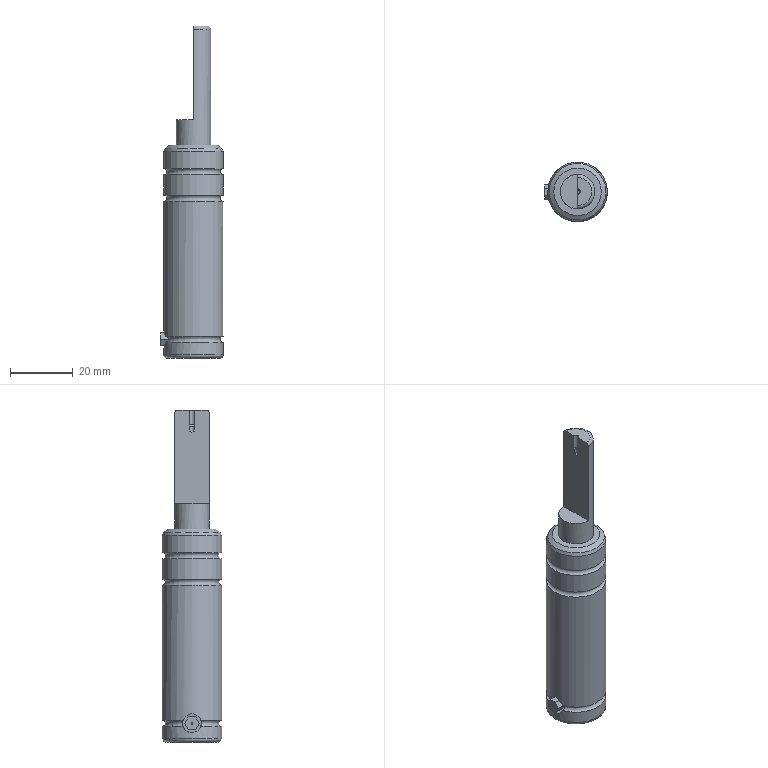Part | NX | features 1 2 | 1 solid | 36 faces | box 20 x 19 x 106 mm | volume 20839 mm3 | plane 14 | cylinder 11 | cone 6 | torus 5 | commonest cylinder face diameters 19 x4 6 x2 0.6 x1 1.558 x1 1.833 x1 5.1 x1
STEP:
#1=CARTESIAN_POINT('',(570.431,-100.172,-102.5));
#2=VERTEX_POINT('',#1);
#3=CARTESIAN_POINT('',(570.431,-100.172,-100.5));
#4=VERTEX_POINT('',#3);
#5=CARTESIAN_POINT('',(570.431,-100.172,-102.5));
#6=CARTESIAN_POINT('',(570.711,-100.172,-102.5));
#7=CARTESIAN_POINT('',(571.253,-100.089,-102.303));
#8=CARTESIAN_POINT('',(571.694,-99.956,-101.501));
#9=CARTESIAN_POINT('',(571.254,-100.089,-100.697));
#10=CARTESIAN_POINT('',(570.711,-100.172,-100.5));
#11=CARTESIAN_POINT('',(570.431,-100.172,-100.5));
#12=B_SPLINE_CURVE_WITH_KNOTS('',3,(#5,#6,#7,#8,#9,#10,#11),.UNSPECIFIED.,.F.,.F.,(4,1,1,1,4),(0.,0.0008273,0.001655,0.002482,0.003309),.UNSPECIFIED.);
#13=EDGE_CURVE('',#2,#4,#12,.T.);
#14=ORIENTED_EDGE('',*,*,#13,.T.);
#15=CARTESIAN_POINT('',(570.431,-105.828,-100.5));
#16=VERTEX_POINT('',#15);
#17=CARTESIAN_POINT('',(579.5,-103.,-100.5));
#18=DIRECTION('',(0.,0.,1.));
#19=DIRECTION('',(-1.,0.,0.));
#20=AXIS2_PLACEMENT_3D('',#17,#18,#19);
#21=CIRCLE('',#20,9.5);
#22=EDGE_CURVE('',#16,#4,#21,.T.);
#23=ORIENTED_EDGE('',*,*,#22,.F.);
#24=CARTESIAN_POINT('',(570.431,-105.828,-102.5));
#25=VERTEX_POINT('',#24);
#26=CARTESIAN_POINT('',(570.431,-105.828,-100.5));
#27=CARTESIAN_POINT('',(570.711,-105.828,-100.5));
#28=CARTESIAN_POINT('',(571.253,-105.911,-100.697));
#29=CARTESIAN_POINT('',(571.694,-106.044,-101.499));
#30=CARTESIAN_POINT('',(571.254,-105.911,-102.303));
#31=CARTESIAN_POINT('',(570.711,-105.828,-102.5));
#32=CARTESIAN_POINT('',(570.431,-105.828,-102.5));
#33=B_SPLINE_CURVE_WITH_KNOTS('',3,(#26,#27,#28,#29,#30,#31,#32),.UNSPECIFIED.,.F.,.F.,(4,1,1,1,4),(-0.001658,-0.0008295,-0.000000739,0.000828,0.001657),.UNSPECIFIED.);
#34=EDGE_CURVE('',#16,#25,#33,.T.);
#35=ORIENTED_EDGE('',*,*,#34,.T.);
#36=CARTESIAN_POINT('',(579.5,-103.,-102.5));
#37=DIRECTION('',(0.,0.,-1.));
#38=DIRECTION('',(-1.,0.,0.));
#39=AXIS2_PLACEMENT_3D('',#36,#37,#38);
#40=CIRCLE('',#39,9.5);
#41=EDGE_CURVE('',#2,#25,#40,.T.);
#42=ORIENTED_EDGE('',*,*,#41,.F.);
#43=EDGE_LOOP('',(#14,#23,#35,#42));
#44=FACE_BOUND('',#43,.T.);
#45=CARTESIAN_POINT('',(579.5,-103.,-101.5));
#46=DIRECTION('',(0.,0.,1.));
#47=DIRECTION('',(1.,0.,0.));
#48=AXIS2_PLACEMENT_3D('',#45,#46,#47);
#49=TOROIDAL_SURFACE('',#48,9.5,1.);
#50=ADVANCED_FACE('',(#44),#49,.F.);
#51=CARTESIAN_POINT('',(570.,-103.,-55.5));
#52=VERTEX_POINT('',#51);
#53=CARTESIAN_POINT('',(579.5,-103.,-55.5));
#54=DIRECTION('',(0.,0.,1.));
#55=DIRECTION('',(-1.,0.,0.));
#56=AXIS2_PLACEMENT_3D('',#53,#54,#55);
#57=CIRCLE('',#56,9.5);
#58=EDGE_CURVE('',#52,#52,#57,.T.);
#59=ORIENTED_EDGE('',*,*,#58,.F.);
#60=EDGE_LOOP('',(#59));
#61=FACE_BOUND('',#60,.T.);
#62=CARTESIAN_POINT('',(570.,-103.,-57.5));
#63=VERTEX_POINT('',#62);
#64=CARTESIAN_POINT('',(579.5,-103.,-57.5));
#65=DIRECTION('',(0.,0.,-1.));
#66=DIRECTION('',(-1.,0.,0.));
#67=AXIS2_PLACEMENT_3D('',#64,#65,#66);
#68=CIRCLE('',#67,9.5);
#69=EDGE_CURVE('',#63,#63,#68,.T.);
#70=ORIENTED_EDGE('',*,*,#69,.F.);
#71=EDGE_LOOP('',(#70));
#72=FACE_BOUND('',#71,.T.);
#73=CARTESIAN_POINT('',(579.5,-103.,-56.5));
#74=DIRECTION('',(0.,0.,1.));
#75=DIRECTION('',(1.,0.,0.));
#76=AXIS2_PLACEMENT_3D('',#73,#74,#75);
#77=TOROIDAL_SURFACE('',#76,9.5,1.);
#78=ADVANCED_FACE('',(#61,#72),#77,.F.);
#79=CARTESIAN_POINT('',(570.,-103.,-47.));
#80=VERTEX_POINT('',#79);
#81=CARTESIAN_POINT('',(579.5,-103.,-47.));
#82=DIRECTION('',(0.,0.,1.));
#83=DIRECTION('',(-1.,0.,0.));
#84=AXIS2_PLACEMENT_3D('',#81,#82,#83);
#85=CIRCLE('',#84,9.5);
#86=EDGE_CURVE('',#80,#80,#85,.T.);
#87=ORIENTED_EDGE('',*,*,#86,.F.);
#88=EDGE_LOOP('',(#87));
#89=FACE_BOUND('',#88,.T.);
#90=CARTESIAN_POINT('',(570.,-103.,-49.));
#91=VERTEX_POINT('',#90);
#92=CARTESIAN_POINT('',(579.5,-103.,-49.));
#93=DIRECTION('',(0.,0.,-1.));
#94=DIRECTION('',(-1.,0.,0.));
#95=AXIS2_PLACEMENT_3D('',#92,#93,#94);
#96=CIRCLE('',#95,9.5);
#97=EDGE_CURVE('',#91,#91,#96,.T.);
#98=ORIENTED_EDGE('',*,*,#97,.F.);
#99=EDGE_LOOP('',(#98));
#100=FACE_BOUND('',#99,.T.);
#101=CARTESIAN_POINT('',(579.5,-103.,-48.));
#102=DIRECTION('',(0.,0.,1.));
#103=DIRECTION('',(1.,0.,0.));
#104=AXIS2_PLACEMENT_3D('',#101,#102,#103);
#105=TOROIDAL_SURFACE('',#104,9.5,1.);
#106=ADVANCED_FACE('',(#89,#100),#105,.F.);
#107=ORIENTED_EDGE('',*,*,#86,.T.);
#108=EDGE_LOOP('',(#107));
#109=FACE_BOUND('',#108,.T.);
#110=CARTESIAN_POINT('',(570.,-103.,-41.5));
#111=VERTEX_POINT('',#110);
#112=CARTESIAN_POINT('',(579.5,-103.,-41.5));
#113=DIRECTION('',(0.,0.,1.));
#114=DIRECTION('',(-1.,0.,0.));
#115=AXIS2_PLACEMENT_3D('',#112,#113,#114);
#116=CIRCLE('',#115,9.5);
#117=EDGE_CURVE('',#111,#111,#116,.T.);
#118=ORIENTED_EDGE('',*,*,#117,.F.);
#119=EDGE_LOOP('',(#118));
#120=FACE_BOUND('',#119,.T.);
#121=CARTESIAN_POINT('',(579.5,-103.,-74.5));
#122=DIRECTION('',(0.,0.,1.));
#123=DIRECTION('',(1.,0.,0.));
#124=AXIS2_PLACEMENT_3D('',#121,#122,#123);
#125=CYLINDRICAL_SURFACE('',#124,9.5);
#126=ADVANCED_FACE('',(#109,#120),#125,.T.);
#127=ORIENTED_EDGE('',*,*,#117,.T.);
#128=EDGE_LOOP('',(#127));
#129=FACE_BOUND('',#128,.T.);
#130=CARTESIAN_POINT('',(570.452,-103.,-40.5));
#131=VERTEX_POINT('',#130);
#132=CARTESIAN_POINT('',(579.5,-103.,-40.5));
#133=DIRECTION('',(0.,0.,1.));
#134=DIRECTION('',(-1.,0.,0.));
#135=AXIS2_PLACEMENT_3D('',#132,#133,#134);
#136=CIRCLE('',#135,9.048);
#137=EDGE_CURVE('',#131,#131,#136,.T.);
#138=ORIENTED_EDGE('',*,*,#137,.F.);
#139=EDGE_LOOP('',(#138));
#140=FACE_BOUND('',#139,.T.);
#141=CARTESIAN_POINT('',(579.5,-103.,-41.));
#142=DIRECTION('',(0.,0.,-1.));
#143=DIRECTION('',(1.,0.,0.));
#144=AXIS2_PLACEMENT_3D('',#141,#142,#143);
#145=CONICAL_SURFACE('',#144,9.274,0.4248);
#146=ADVANCED_FACE('',(#129,#140),#145,.T.);
#147=ORIENTED_EDGE('',*,*,#137,.T.);
#148=EDGE_LOOP('',(#147));
#149=FACE_BOUND('',#148,.T.);
#150=CARTESIAN_POINT('',(571.9,-103.,-39.5));
#151=VERTEX_POINT('',#150);
#152=CARTESIAN_POINT('',(579.5,-103.,-39.5));
#153=DIRECTION('',(0.,0.,1.));
#154=DIRECTION('',(-1.,0.,0.));
#155=AXIS2_PLACEMENT_3D('',#152,#153,#154);
#156=CIRCLE('',#155,7.6);
#157=EDGE_CURVE('',#151,#151,#156,.T.);
#158=ORIENTED_EDGE('',*,*,#157,.F.);
#159=EDGE_LOOP('',(#158));
#160=FACE_BOUND('',#159,.T.);
#161=CARTESIAN_POINT('',(579.5,-103.,-40.));
#162=DIRECTION('',(0.,0.,-1.));
#163=DIRECTION('',(1.,0.,0.));
#164=AXIS2_PLACEMENT_3D('',#161,#162,#163);
#165=CONICAL_SURFACE('',#164,8.324,0.9663);
#166=ADVANCED_FACE('',(#149,#160),#165,.T.);
#167=ORIENTED_EDGE('',*,*,#22,.T.);
#168=CARTESIAN_POINT('',(570.431,-100.172,-100.5));
#169=CARTESIAN_POINT('',(570.366,-100.379,-99.913));
#170=CARTESIAN_POINT('',(570.138,-101.142,-98.904));
#171=CARTESIAN_POINT('',(569.931,-103.001,-98.299));
#172=CARTESIAN_POINT('',(570.136,-104.85,-98.899));
#173=CARTESIAN_POINT('',(570.366,-105.621,-99.913));
#174=CARTESIAN_POINT('',(570.431,-105.828,-100.5));
#175=B_SPLINE_CURVE_WITH_KNOTS('',3,(#168,#169,#170,#171,#172,#173,#174),.UNSPECIFIED.,.F.,.F.,(4,1,1,1,4),(-0.003701,-0.001851,-0.000000566,0.00185,0.0037),.UNSPECIFIED.);
#176=EDGE_CURVE('',#4,#16,#175,.T.);
#177=ORIENTED_EDGE('',*,*,#176,.T.);
#178=EDGE_LOOP('',(#167,#177));
#179=FACE_BOUND('',#178,.T.);
#180=ORIENTED_EDGE('',*,*,#69,.T.);
#181=EDGE_LOOP('',(#180));
#182=FACE_BOUND('',#181,.T.);
#183=CARTESIAN_POINT('',(579.5,-103.,-74.5));
#184=DIRECTION('',(0.,0.,1.));
#185=DIRECTION('',(1.,0.,0.));
#186=AXIS2_PLACEMENT_3D('',#183,#184,#185);
#187=CYLINDRICAL_SURFACE('',#186,9.5);
#188=ADVANCED_FACE('',(#179,#182),#187,.T.);
#189=ORIENTED_EDGE('',*,*,#58,.T.);
#190=EDGE_LOOP('',(#189));
#191=FACE_BOUND('',#190,.T.);
#192=ORIENTED_EDGE('',*,*,#97,.T.);
#193=EDGE_LOOP('',(#192));
#194=FACE_BOUND('',#193,.T.);
#195=CARTESIAN_POINT('',(579.5,-103.,-74.5));
#196=DIRECTION('',(0.,0.,1.));
#197=DIRECTION('',(1.,0.,0.));
#198=AXIS2_PLACEMENT_3D('',#195,#196,#197);
#199=CYLINDRICAL_SURFACE('',#198,9.5);
#200=ADVANCED_FACE('',(#191,#194),#199,.T.);
#201=CARTESIAN_POINT('',(579.5,-102.083,-6.25));
#202=VERTEX_POINT('',#201);
#203=CARTESIAN_POINT('',(579.5,-103.917,-6.25));
#204=VERTEX_POINT('',#203);
#205=CARTESIAN_POINT('',(579.5,-103.,-6.25));
#206=DIRECTION('',(0.,0.,-1.));
#207=DIRECTION('',(-1.,0.,0.));
#208=AXIS2_PLACEMENT_3D('',#205,#206,#207);
#209=CIRCLE('',#208,0.9167);
#210=EDGE_CURVE('',#202,#204,#209,.T.);
#211=ORIENTED_EDGE('',*,*,#210,.T.);
#212=CARTESIAN_POINT('',(579.5,-103.917,-1.5));
#213=VERTEX_POINT('',#212);
#214=CARTESIAN_POINT('',(579.5,-103.917,-3.875));
#215=DIRECTION('',(0.,0.,-1.));
#216=VECTOR('',#215,1000.);
#217=LINE('',#214,#216);
#218=EDGE_CURVE('',#204,#213,#217,.F.);
#219=ORIENTED_EDGE('',*,*,#218,.T.);
#220=CARTESIAN_POINT('',(579.5,-102.083,-1.5));
#221=VERTEX_POINT('',#220);
#222=CARTESIAN_POINT('',(579.5,-103.,-1.5));
#223=DIRECTION('',(0.,0.,-1.));
#224=DIRECTION('',(-1.,0.,0.));
#225=AXIS2_PLACEMENT_3D('',#222,#223,#224);
#226=CIRCLE('',#225,0.9167);
#227=EDGE_CURVE('',#221,#213,#226,.T.);
#228=ORIENTED_EDGE('',*,*,#227,.F.);
#229=CARTESIAN_POINT('',(579.5,-102.083,-3.875));
#230=DIRECTION('',(0.,0.,-1.));
#231=VECTOR('',#230,1000.);
#232=LINE('',#229,#231);
#233=EDGE_CURVE('',#221,#202,#232,.T.);
#234=ORIENTED_EDGE('',*,*,#233,.T.);
#235=EDGE_LOOP('',(#211,#219,#228,#234));
#236=FACE_BOUND('',#235,.T.);
#237=CARTESIAN_POINT('',(579.5,-103.,-3.875));
#238=DIRECTION('',(0.,0.,-1.));
#239=DIRECTION('',(1.,0.,0.));
#240=AXIS2_PLACEMENT_3D('',#237,#238,#239);
#241=CYLINDRICAL_SURFACE('',#240,0.9167);
#242=ADVANCED_FACE('',(#236),#241,.F.);
#243=ORIENTED_EDGE('',*,*,#210,.F.);
#244=CARTESIAN_POINT('',(579.5,-102.221,-6.75));
#245=VERTEX_POINT('',#244);
#246=CARTESIAN_POINT('',(579.5,-103.,-9.583));
#247=DIRECTION('',(0.,0.2652,0.9642));
#248=VECTOR('',#247,1000.);
#249=LINE('',#246,#248);
#250=EDGE_CURVE('',#202,#245,#249,.F.);
#251=ORIENTED_EDGE('',*,*,#250,.T.);
#252=CARTESIAN_POINT('',(579.5,-103.779,-6.75));
#253=VERTEX_POINT('',#252);
#254=CARTESIAN_POINT('',(579.5,-103.,-6.75));
#255=DIRECTION('',(0.,0.,-1.));
#256=DIRECTION('',(-1.,0.,0.));
#257=AXIS2_PLACEMENT_3D('',#254,#255,#256);
#258=CIRCLE('',#257,0.7792);
#259=EDGE_CURVE('',#245,#253,#258,.T.);
#260=ORIENTED_EDGE('',*,*,#259,.T.);
#261=CARTESIAN_POINT('',(579.5,-103.,-9.583));
#262=DIRECTION('',(0.,0.2652,-0.9642));
#263=VECTOR('',#262,1000.);
#264=LINE('',#261,#263);
#265=EDGE_CURVE('',#253,#204,#264,.F.);
#266=ORIENTED_EDGE('',*,*,#265,.T.);
#267=EDGE_LOOP('',(#243,#251,#260,#266));
#268=FACE_BOUND('',#267,.T.);
#269=CARTESIAN_POINT('',(579.5,-103.,-6.5));
#270=DIRECTION('',(0.,0.,1.));
#271=DIRECTION('',(1.,0.,0.));
#272=AXIS2_PLACEMENT_3D('',#269,#270,#271);
#273=CONICAL_SURFACE('',#272,0.8479,0.2684);
#274=ADVANCED_FACE('',(#268),#273,.F.);
#275=CARTESIAN_POINT('',(579.5,-102.221,-8.25));
#276=VERTEX_POINT('',#275);
#277=CARTESIAN_POINT('',(579.5,-103.779,-8.25));
#278=VERTEX_POINT('',#277);
#279=CARTESIAN_POINT('',(579.5,-103.,-8.25));
#280=DIRECTION('',(0.,0.,-1.));
#281=DIRECTION('',(-1.,0.,0.));
#282=AXIS2_PLACEMENT_3D('',#279,#280,#281);
#283=CIRCLE('',#282,0.7792);
#284=EDGE_CURVE('',#276,#278,#283,.T.);
#285=ORIENTED_EDGE('',*,*,#284,.T.);
#286=CARTESIAN_POINT('',(579.5,-103.779,-7.5));
#287=DIRECTION('',(0.,0.,-1.));
#288=VECTOR('',#287,1000.);
#289=LINE('',#286,#288);
#290=EDGE_CURVE('',#278,#253,#289,.F.);
#291=ORIENTED_EDGE('',*,*,#290,.T.);
#292=ORIENTED_EDGE('',*,*,#259,.F.);
#293=CARTESIAN_POINT('',(579.5,-102.221,-7.5));
#294=DIRECTION('',(0.,0.,-1.));
#295=VECTOR('',#294,1000.);
#296=LINE('',#293,#295);
#297=EDGE_CURVE('',#245,#276,#296,.T.);
#298=ORIENTED_EDGE('',*,*,#297,.T.);
#299=EDGE_LOOP('',(#285,#291,#292,#298));
#300=FACE_BOUND('',#299,.T.);
#301=CARTESIAN_POINT('',(579.5,-103.,-7.5));
#302=DIRECTION('',(0.,0.,-1.));
#303=DIRECTION('',(1.,0.,0.));
#304=AXIS2_PLACEMENT_3D('',#301,#302,#303);
#305=CYLINDRICAL_SURFACE('',#304,0.7792);
#306=ADVANCED_FACE('',(#300),#305,.F.);
#307=ORIENTED_EDGE('',*,*,#284,.F.);
#308=CARTESIAN_POINT('',(579.5,-103.,-8.718));
#309=VERTEX_POINT('',#308);
#310=CARTESIAN_POINT('',(579.5,-103.,-8.718));
#311=DIRECTION('',(0.,0.8572,0.515));
#312=VECTOR('',#311,1000.);
#313=LINE('',#310,#312);
#314=EDGE_CURVE('',#276,#309,#313,.F.);
#315=ORIENTED_EDGE('',*,*,#314,.T.);
#316=CARTESIAN_POINT('',(579.5,-103.,-8.718));
#317=DIRECTION('',(0.,0.8572,-0.515));
#318=VECTOR('',#317,1000.);
#319=LINE('',#316,#318);
#320=EDGE_CURVE('',#309,#278,#319,.F.);
#321=ORIENTED_EDGE('',*,*,#320,.T.);
#322=EDGE_LOOP('',(#307,#315,#321));
#323=FACE_BOUND('',#322,.T.);
#324=CARTESIAN_POINT('',(579.5,-103.,-8.484));
#325=DIRECTION('',(0.,0.,1.));
#326=DIRECTION('',(1.,0.,0.));
#327=AXIS2_PLACEMENT_3D('',#324,#325,#326);
#328=CONICAL_SURFACE('',#327,0.3896,1.03);
#329=ADVANCED_FACE('',(#323),#328,.F.);
#330=CARTESIAN_POINT('',(576.5,-103.,-101.5));
#331=VERTEX_POINT('',#330);
#332=CARTESIAN_POINT('',(579.5,-103.,-101.5));
#333=DIRECTION('',(0.,0.,1.));
#334=DIRECTION('',(-1.,0.,0.));
#335=AXIS2_PLACEMENT_3D('',#332,#333,#334);
#336=CIRCLE('',#335,3.);
#337=EDGE_CURVE('',#331,#331,#336,.T.);
#338=ORIENTED_EDGE('',*,*,#337,.T.);
#339=EDGE_LOOP('',(#338));
#340=FACE_BOUND('',#339,.T.);
#341=CARTESIAN_POINT('',(576.5,-103.,-107.5));
#342=VERTEX_POINT('',#341);
#343=CARTESIAN_POINT('',(579.5,-103.,-107.5));
#344=DIRECTION('',(0.,0.,1.));
#345=DIRECTION('',(-1.,0.,0.));
#346=AXIS2_PLACEMENT_3D('',#343,#344,#345);
#347=CIRCLE('',#346,3.);
#348=EDGE_CURVE('',#342,#342,#347,.T.);
#349=ORIENTED_EDGE('',*,*,#348,.F.);
#350=EDGE_LOOP('',(#349));
#351=FACE_BOUND('',#350,.T.);
#352=CARTESIAN_POINT('',(579.5,-103.,-104.5));
#353=DIRECTION('',(0.,0.,1.));
#354=DIRECTION('',(1.,0.,0.));
#355=AXIS2_PLACEMENT_3D('',#352,#353,#354);
#356=CYLINDRICAL_SURFACE('',#355,3.);
#357=ADVANCED_FACE('',(#340,#351),#356,.F.);
#358=CARTESIAN_POINT('',(576.95,-103.,-101.));
#359=VERTEX_POINT('',#358);
#360=CARTESIAN_POINT('',(579.5,-103.,-101.));
#361=DIRECTION('',(0.,0.,1.));
#362=DIRECTION('',(-1.,0.,0.));
#363=AXIS2_PLACEMENT_3D('',#360,#361,#362);
#364=CIRCLE('',#363,2.55);
#365=EDGE_CURVE('',#359,#359,#364,.T.);
#366=ORIENTED_EDGE('',*,*,#365,.T.);
#367=EDGE_LOOP('',(#366));
#368=FACE_BOUND('',#367,.T.);
#369=ORIENTED_EDGE('',*,*,#337,.F.);
#370=EDGE_LOOP('',(#369));
#371=FACE_BOUND('',#370,.T.);
#372=CARTESIAN_POINT('',(579.5,-103.,-101.25));
#373=DIRECTION('',(0.,0.,-1.));
#374=DIRECTION('',(1.,0.,0.));
#375=AXIS2_PLACEMENT_3D('',#372,#373,#374);
#376=CONICAL_SURFACE('',#375,2.775,0.7328);
#377=ADVANCED_FACE('',(#368,#371),#376,.F.);
#378=CARTESIAN_POINT('',(576.95,-103.,-99.5));
#379=VERTEX_POINT('',#378);
#380=CARTESIAN_POINT('',(579.5,-103.,-99.5));
#381=DIRECTION('',(0.,0.,1.));
#382=DIRECTION('',(-1.,0.,0.));
#383=AXIS2_PLACEMENT_3D('',#380,#381,#382);
#384=CIRCLE('',#383,2.55);
#385=EDGE_CURVE('',#379,#379,#384,.T.);
#386=ORIENTED_EDGE('',*,*,#385,.T.);
#387=EDGE_LOOP('',(#386));
#388=FACE_BOUND('',#387,.T.);
#389=ORIENTED_EDGE('',*,*,#365,.F.);
#390=EDGE_LOOP('',(#389));
#391=FACE_BOUND('',#390,.T.);
#392=CARTESIAN_POINT('',(579.5,-103.,-100.25));
#393=DIRECTION('',(0.,0.,1.));
#394=DIRECTION('',(1.,0.,0.));
#395=AXIS2_PLACEMENT_3D('',#392,#393,#394);
#396=CYLINDRICAL_SURFACE('',#395,2.55);
#397=ADVANCED_FACE('',(#388,#391),#396,.F.);
#398=ORIENTED_EDGE('',*,*,#385,.F.);
#399=EDGE_LOOP('',(#398));
#400=FACE_BOUND('',#399,.T.);
#401=CARTESIAN_POINT('',(579.5,-103.,-97.968));
#402=VERTEX_POINT('',#401);
#403=VERTEX_LOOP('',#402);
#404=FACE_BOUND('',#403,.T.);
#405=CARTESIAN_POINT('',(579.5,-103.,-98.734));
#406=DIRECTION('',(0.,0.,-1.));
#407=DIRECTION('',(1.,0.,0.));
#408=AXIS2_PLACEMENT_3D('',#405,#406,#407);
#409=CONICAL_SURFACE('',#408,1.275,1.03);
#410=ADVANCED_FACE('',(#400,#404),#409,.F.);
#411=CARTESIAN_POINT('',(579.5,-97.5,-2.5));
#412=VERTEX_POINT('',#411);
#413=CARTESIAN_POINT('',(579.5,-97.5,-31.5));
#414=VERTEX_POINT('',#413);
#415=CARTESIAN_POINT('',(579.5,-97.5,-20.5));
#416=DIRECTION('',(0.,0.,1.));
#417=VECTOR('',#416,1000.);
#418=LINE('',#415,#417);
#419=EDGE_CURVE('',#412,#414,#418,.F.);
#420=ORIENTED_EDGE('',*,*,#419,.F.);
#421=CARTESIAN_POINT('',(579.5,-108.5,-2.5));
#422=VERTEX_POINT('',#421);
#423=CARTESIAN_POINT('',(579.5,-103.,-2.5));
#424=DIRECTION('',(0.,0.,1.));
#425=DIRECTION('',(1.,0.,0.));
#426=AXIS2_PLACEMENT_3D('',#423,#424,#425);
#427=CIRCLE('',#426,5.5);
#428=EDGE_CURVE('',#422,#412,#427,.T.);
#429=ORIENTED_EDGE('',*,*,#428,.F.);
#430=CARTESIAN_POINT('',(579.5,-108.5,-31.5));
#431=VERTEX_POINT('',#430);
#432=CARTESIAN_POINT('',(579.5,-108.5,-20.5));
#433=DIRECTION('',(0.,0.,1.));
#434=VECTOR('',#433,1000.);
#435=LINE('',#432,#434);
#436=EDGE_CURVE('',#431,#422,#435,.T.);
#437=ORIENTED_EDGE('',*,*,#436,.F.);
#438=CARTESIAN_POINT('',(579.5,-103.,-31.5));
#439=DIRECTION('',(0.,0.,-1.));
#440=DIRECTION('',(-1.,0.,0.));
#441=AXIS2_PLACEMENT_3D('',#438,#439,#440);
#442=CIRCLE('',#441,5.5);
#443=EDGE_CURVE('',#414,#431,#442,.F.);
#444=ORIENTED_EDGE('',*,*,#443,.F.);
#445=EDGE_LOOP('',(#420,#429,#437,#444));
#446=FACE_BOUND('',#445,.T.);
#447=CARTESIAN_POINT('',(574.,-103.,-39.5));
#448=VERTEX_POINT('',#447);
#449=CARTESIAN_POINT('',(579.5,-103.,-39.5));
#450=DIRECTION('',(0.,0.,-1.));
#451=DIRECTION('',(-1.,0.,0.));
#452=AXIS2_PLACEMENT_3D('',#449,#450,#451);
#453=CIRCLE('',#452,5.5);
#454=EDGE_CURVE('',#448,#448,#453,.T.);
#455=ORIENTED_EDGE('',*,*,#454,.F.);
#456=EDGE_LOOP('',(#455));
#457=FACE_BOUND('',#456,.T.);
#458=CARTESIAN_POINT('',(579.5,-103.,-20.5));
#459=DIRECTION('',(0.,0.,1.));
#460=DIRECTION('',(1.,0.,0.));
#461=AXIS2_PLACEMENT_3D('',#458,#459,#460);
#462=CYLINDRICAL_SURFACE('',#461,5.5);
#463=ADVANCED_FACE('',(#446,#457),#462,.T.);
#464=CARTESIAN_POINT('',(579.5,-98.5,-1.5));
#465=VERTEX_POINT('',#464);
#466=CARTESIAN_POINT('',(579.5,-98.5,-2.5));
#467=DIRECTION('',(1.,0.,0.));
#468=DIRECTION('',(0.,0.,-1.));
#469=AXIS2_PLACEMENT_3D('',#466,#467,#468);
#470=CIRCLE('',#469,1.);
#471=EDGE_CURVE('',#465,#412,#470,.F.);
#472=ORIENTED_EDGE('',*,*,#471,.F.);
#473=CARTESIAN_POINT('',(579.5,-107.5,-1.5));
#474=VERTEX_POINT('',#473);
#475=CARTESIAN_POINT('',(579.5,-103.,-1.5));
#476=DIRECTION('',(0.,0.,-1.));
#477=DIRECTION('',(1.,0.,0.));
#478=AXIS2_PLACEMENT_3D('',#475,#476,#477);
#479=CIRCLE('',#478,4.5);
#480=EDGE_CURVE('',#465,#474,#479,.T.);
#481=ORIENTED_EDGE('',*,*,#480,.T.);
#482=CARTESIAN_POINT('',(579.5,-107.5,-2.5));
#483=DIRECTION('',(1.,0.,0.));
#484=DIRECTION('',(0.,0.,-1.));
#485=AXIS2_PLACEMENT_3D('',#482,#483,#484);
#486=CIRCLE('',#485,1.);
#487=EDGE_CURVE('',#422,#474,#486,.F.);
#488=ORIENTED_EDGE('',*,*,#487,.F.);
#489=ORIENTED_EDGE('',*,*,#428,.T.);
#490=EDGE_LOOP('',(#472,#481,#488,#489));
#491=FACE_BOUND('',#490,.T.);
#492=CARTESIAN_POINT('',(579.5,-103.,-2.5));
#493=DIRECTION('',(0.,0.,1.));
#494=DIRECTION('',(1.,0.,0.));
#495=AXIS2_PLACEMENT_3D('',#492,#493,#494);
#496=TOROIDAL_SURFACE('',#495,4.5,1.);
#497=ADVANCED_FACE('',(#491),#496,.T.);
#498=CARTESIAN_POINT('',(589.,-103.,-106.5));
#499=VERTEX_POINT('',#498);
#500=CARTESIAN_POINT('',(579.5,-103.,-106.5));
#501=DIRECTION('',(0.,0.,-1.));
#502=DIRECTION('',(1.,0.,0.));
#503=AXIS2_PLACEMENT_3D('',#500,#501,#502);
#504=CIRCLE('',#503,9.5);
#505=EDGE_CURVE('',#499,#499,#504,.T.);
#506=ORIENTED_EDGE('',*,*,#505,.T.);
#507=EDGE_LOOP('',(#506));
#508=FACE_BOUND('',#507,.T.);
#509=CARTESIAN_POINT('',(588.,-103.,-107.5));
#510=VERTEX_POINT('',#509);
#511=CARTESIAN_POINT('',(579.5,-103.,-107.5));
#512=DIRECTION('',(0.,0.,1.));
#513=DIRECTION('',(1.,0.,0.));
#514=AXIS2_PLACEMENT_3D('',#511,#512,#513);
#515=CIRCLE('',#514,8.5);
#516=EDGE_CURVE('',#510,#510,#515,.T.);
#517=ORIENTED_EDGE('',*,*,#516,.T.);
#518=EDGE_LOOP('',(#517));
#519=FACE_BOUND('',#518,.T.);
#520=CARTESIAN_POINT('',(579.5,-103.,-106.5));
#521=DIRECTION('',(0.,0.,-1.));
#522=DIRECTION('',(-1.,0.,0.));
#523=AXIS2_PLACEMENT_3D('',#520,#521,#522);
#524=TOROIDAL_SURFACE('',#523,8.5,1.);
#525=ADVANCED_FACE('',(#508,#519),#524,.T.);
#526=ORIENTED_EDGE('',*,*,#505,.F.);
#527=EDGE_LOOP('',(#526));
#528=FACE_BOUND('',#527,.T.);
#529=CARTESIAN_POINT('',(570.431,-105.828,-102.5));
#530=CARTESIAN_POINT('',(570.366,-105.621,-103.087));
#531=CARTESIAN_POINT('',(570.138,-104.858,-104.096));
#532=CARTESIAN_POINT('',(569.931,-102.999,-104.701));
#533=CARTESIAN_POINT('',(570.136,-101.15,-104.101));
#534=CARTESIAN_POINT('',(570.366,-100.379,-103.087));
#535=CARTESIAN_POINT('',(570.431,-100.172,-102.5));
#536=B_SPLINE_CURVE_WITH_KNOTS('',3,(#529,#530,#531,#532,#533,#534,#535),.UNSPECIFIED.,.F.,.F.,(4,1,1,1,4),(0.,0.00185,0.0037,0.005549,0.007399),.UNSPECIFIED.);
#537=EDGE_CURVE('',#25,#2,#536,.T.);
#538=ORIENTED_EDGE('',*,*,#537,.T.);
#539=ORIENTED_EDGE('',*,*,#41,.T.);
#540=EDGE_LOOP('',(#538,#539));
#541=FACE_BOUND('',#540,.T.);
#542=CARTESIAN_POINT('',(579.5,-103.,-74.5));
#543=DIRECTION('',(0.,0.,1.));
#544=DIRECTION('',(1.,0.,0.));
#545=AXIS2_PLACEMENT_3D('',#542,#543,#544);
#546=CYLINDRICAL_SURFACE('',#545,9.5);
#547=ADVANCED_FACE('',(#528,#541),#546,.T.);
#548=CARTESIAN_POINT('',(574.,-103.,-98.5));
#549=VERTEX_POINT('',#548);
#550=CARTESIAN_POINT('',(574.,-103.,-101.5));
#551=DIRECTION('',(1.,0.,0.));
#552=DIRECTION('',(0.,0.,1.));
#553=AXIS2_PLACEMENT_3D('',#550,#551,#552);
#554=CIRCLE('',#553,3.);
#555=EDGE_CURVE('',#549,#549,#554,.T.);
#556=ORIENTED_EDGE('',*,*,#555,.T.);
#557=EDGE_LOOP('',(#556));
#558=FACE_BOUND('',#557,.T.);
#559=ORIENTED_EDGE('',*,*,#176,.F.);
#560=ORIENTED_EDGE('',*,*,#13,.F.);
#561=ORIENTED_EDGE('',*,*,#537,.F.);
#562=ORIENTED_EDGE('',*,*,#34,.F.);
#563=EDGE_LOOP('',(#559,#560,#561,#562));
#564=FACE_BOUND('',#563,.T.);
#565=CARTESIAN_POINT('',(572.,-103.,-101.5));
#566=DIRECTION('',(1.,0.,0.));
#567=DIRECTION('',(0.,0.,-1.));
#568=AXIS2_PLACEMENT_3D('',#565,#566,#567);
#569=CYLINDRICAL_SURFACE('',#568,3.);
#570=ADVANCED_FACE('',(#558,#564),#569,.F.);
#571=CARTESIAN_POINT('',(574.,-103.,-101.2));
#572=VERTEX_POINT('',#571);
#573=CARTESIAN_POINT('',(574.,-103.,-101.5));
#574=DIRECTION('',(1.,0.,0.));
#575=DIRECTION('',(0.,0.,1.));
#576=AXIS2_PLACEMENT_3D('',#573,#574,#575);
#577=CIRCLE('',#576,0.3);
#578=EDGE_CURVE('',#572,#572,#577,.T.);
#579=ORIENTED_EDGE('',*,*,#578,.T.);
#580=EDGE_LOOP('',(#579));
#581=FACE_BOUND('',#580,.T.);
#582=CARTESIAN_POINT('',(569.,-103.,-101.2));
#583=VERTEX_POINT('',#582);
#584=CARTESIAN_POINT('',(569.,-103.,-101.5));
#585=DIRECTION('',(1.,0.,0.));
#586=DIRECTION('',(0.,0.,1.));
#587=AXIS2_PLACEMENT_3D('',#584,#585,#586);
#588=CIRCLE('',#587,0.3);
#589=EDGE_CURVE('',#583,#583,#588,.T.);
#590=ORIENTED_EDGE('',*,*,#589,.F.);
#591=EDGE_LOOP('',(#590));
#592=FACE_BOUND('',#591,.T.);
#593=CARTESIAN_POINT('',(570.5,-103.,-101.5));
#594=DIRECTION('',(1.,0.,0.));
#595=DIRECTION('',(0.,0.,-1.));
#596=AXIS2_PLACEMENT_3D('',#593,#594,#595);
#597=CYLINDRICAL_SURFACE('',#596,0.3);
#598=ADVANCED_FACE('',(#581,#592),#597,.F.);
#599=ORIENTED_EDGE('',*,*,#578,.F.);
#600=EDGE_LOOP('',(#599));
#601=FACE_BOUND('',#600,.T.);
#602=CARTESIAN_POINT('',(574.,-103.,-101.5));
#603=DIRECTION('',(1.,0.,0.));
#604=DIRECTION('',(0.,0.,-1.));
#605=AXIS2_PLACEMENT_3D('',#602,#603,#604);
#606=PLANE('',#605);
#607=ADVANCED_FACE('',(#601),#606,.F.);
#608=ORIENTED_EDGE('',*,*,#589,.T.);
#609=EDGE_LOOP('',(#608));
#610=FACE_BOUND('',#609,.T.);
#611=CARTESIAN_POINT('',(569.,-104.155,-99.5));
#612=VERTEX_POINT('',#611);
#613=CARTESIAN_POINT('',(569.,-101.845,-99.5));
#614=VERTEX_POINT('',#613);
#615=CARTESIAN_POINT('',(569.,-103.,-99.5));
#616=DIRECTION('',(0.,1.,0.));
#617=VECTOR('',#616,1000.);
#618=LINE('',#615,#617);
#619=EDGE_CURVE('',#612,#614,#618,.T.);
#620=ORIENTED_EDGE('',*,*,#619,.T.);
#621=CARTESIAN_POINT('',(569.,-100.691,-101.5));
#622=VERTEX_POINT('',#621);
#623=CARTESIAN_POINT('',(569.,-101.268,-100.5));
#624=DIRECTION('',(0.,0.5,-0.866));
#625=VECTOR('',#624,1000.);
#626=LINE('',#623,#625);
#627=EDGE_CURVE('',#614,#622,#626,.T.);
#628=ORIENTED_EDGE('',*,*,#627,.T.);
#629=CARTESIAN_POINT('',(569.,-101.845,-103.5));
#630=VERTEX_POINT('',#629);
#631=CARTESIAN_POINT('',(569.,-101.268,-102.5));
#632=DIRECTION('',(0.,-0.5,-0.866));
#633=VECTOR('',#632,1000.);
#634=LINE('',#631,#633);
#635=EDGE_CURVE('',#622,#630,#634,.T.);
#636=ORIENTED_EDGE('',*,*,#635,.T.);
#637=CARTESIAN_POINT('',(569.,-104.155,-103.5));
#638=VERTEX_POINT('',#637);
#639=CARTESIAN_POINT('',(569.,-103.,-103.5));
#640=DIRECTION('',(0.,-1.,0.));
#641=VECTOR('',#640,1000.);
#642=LINE('',#639,#641);
#643=EDGE_CURVE('',#630,#638,#642,.T.);
#644=ORIENTED_EDGE('',*,*,#643,.T.);
#645=CARTESIAN_POINT('',(569.,-105.309,-101.5));
#646=VERTEX_POINT('',#645);
#647=CARTESIAN_POINT('',(569.,-104.732,-102.5));
#648=DIRECTION('',(0.,-0.5,0.866));
#649=VECTOR('',#648,1000.);
#650=LINE('',#647,#649);
#651=EDGE_CURVE('',#638,#646,#650,.T.);
#652=ORIENTED_EDGE('',*,*,#651,.T.);
#653=CARTESIAN_POINT('',(569.,-104.732,-100.5));
#654=DIRECTION('',(0.,0.5,0.866));
#655=VECTOR('',#654,1000.);
#656=LINE('',#653,#655);
#657=EDGE_CURVE('',#646,#612,#656,.T.);
#658=ORIENTED_EDGE('',*,*,#657,.T.);
#659=EDGE_LOOP('',(#620,#628,#636,#644,#652,#658));
#660=FACE_BOUND('',#659,.T.);
#661=CARTESIAN_POINT('',(569.,-103.,-101.5));
#662=DIRECTION('',(-1.,0.,0.));
#663=DIRECTION('',(0.,0.,-1.));
#664=AXIS2_PLACEMENT_3D('',#661,#662,#663);
#665=PLANE('',#664);
#666=ADVANCED_FACE('',(#610,#660),#665,.T.);
#667=CARTESIAN_POINT('',(574.,-105.309,-101.5));
#668=VERTEX_POINT('',#667);
#669=CARTESIAN_POINT('',(571.5,-105.309,-101.5));
#670=DIRECTION('',(1.,0.,0.));
#671=VECTOR('',#670,1000.);
#672=LINE('',#669,#671);
#673=EDGE_CURVE('',#646,#668,#672,.T.);
#674=ORIENTED_EDGE('',*,*,#673,.T.);
#675=CARTESIAN_POINT('',(574.,-104.155,-99.5));
#676=VERTEX_POINT('',#675);
#677=CARTESIAN_POINT('',(574.,-104.732,-100.5));
#678=DIRECTION('',(0.,-0.5,-0.866));
#679=VECTOR('',#678,1000.);
#680=LINE('',#677,#679);
#681=EDGE_CURVE('',#676,#668,#680,.T.);
#682=ORIENTED_EDGE('',*,*,#681,.F.);
#683=CARTESIAN_POINT('',(571.5,-104.155,-99.5));
#684=DIRECTION('',(1.,0.,0.));
#685=VECTOR('',#684,1000.);
#686=LINE('',#683,#685);
#687=EDGE_CURVE('',#612,#676,#686,.T.);
#688=ORIENTED_EDGE('',*,*,#687,.F.);
#689=ORIENTED_EDGE('',*,*,#657,.F.);
#690=EDGE_LOOP('',(#674,#682,#688,#689));
#691=FACE_BOUND('',#690,.T.);
#692=CARTESIAN_POINT('',(571.5,-104.732,-100.5));
#693=DIRECTION('',(0.,0.866,-0.5));
#694=DIRECTION('',(1.,0.,0.));
#695=AXIS2_PLACEMENT_3D('',#692,#693,#694);
#696=PLANE('',#695);
#697=ADVANCED_FACE('',(#691),#696,.F.);
#698=CARTESIAN_POINT('',(574.,-104.155,-103.5));
#699=VERTEX_POINT('',#698);
#700=CARTESIAN_POINT('',(571.5,-104.155,-103.5));
#701=DIRECTION('',(1.,0.,0.));
#702=VECTOR('',#701,1000.);
#703=LINE('',#700,#702);
#704=EDGE_CURVE('',#638,#699,#703,.T.);
#705=ORIENTED_EDGE('',*,*,#704,.T.);
#706=CARTESIAN_POINT('',(574.,-104.732,-102.5));
#707=DIRECTION('',(0.,0.5,-0.866));
#708=VECTOR('',#707,1000.);
#709=LINE('',#706,#708);
#710=EDGE_CURVE('',#668,#699,#709,.T.);
#711=ORIENTED_EDGE('',*,*,#710,.F.);
#712=ORIENTED_EDGE('',*,*,#673,.F.);
#713=ORIENTED_EDGE('',*,*,#651,.F.);
#714=EDGE_LOOP('',(#705,#711,#712,#713));
#715=FACE_BOUND('',#714,.T.);
#716=CARTESIAN_POINT('',(571.5,-104.732,-102.5));
#717=DIRECTION('',(0.,0.866,0.5));
#718=DIRECTION('',(-1.,0.,0.));
#719=AXIS2_PLACEMENT_3D('',#716,#717,#718);
#720=PLANE('',#719);
#721=ADVANCED_FACE('',(#715),#720,.F.);
#722=CARTESIAN_POINT('',(574.,-101.845,-103.5));
#723=VERTEX_POINT('',#722);
#724=CARTESIAN_POINT('',(571.5,-101.845,-103.5));
#725=DIRECTION('',(1.,0.,0.));
#726=VECTOR('',#725,1000.);
#727=LINE('',#724,#726);
#728=EDGE_CURVE('',#630,#723,#727,.T.);
#729=ORIENTED_EDGE('',*,*,#728,.T.);
#730=CARTESIAN_POINT('',(574.,-103.,-103.5));
#731=DIRECTION('',(0.,1.,0.));
#732=VECTOR('',#731,1000.);
#733=LINE('',#730,#732);
#734=EDGE_CURVE('',#699,#723,#733,.T.);
#735=ORIENTED_EDGE('',*,*,#734,.F.);
#736=ORIENTED_EDGE('',*,*,#704,.F.);
#737=ORIENTED_EDGE('',*,*,#643,.F.);
#738=EDGE_LOOP('',(#729,#735,#736,#737));
#739=FACE_BOUND('',#738,.T.);
#740=CARTESIAN_POINT('',(571.5,-103.,-103.5));
#741=DIRECTION('',(0.,0.,1.));
#742=DIRECTION('',(-1.,0.,0.));
#743=AXIS2_PLACEMENT_3D('',#740,#741,#742);
#744=PLANE('',#743);
#745=ADVANCED_FACE('',(#739),#744,.F.);
#746=CARTESIAN_POINT('',(574.,-100.691,-101.5));
#747=VERTEX_POINT('',#746);
#748=CARTESIAN_POINT('',(571.5,-100.691,-101.5));
#749=DIRECTION('',(1.,0.,0.));
#750=VECTOR('',#749,1000.);
#751=LINE('',#748,#750);
#752=EDGE_CURVE('',#622,#747,#751,.T.);
#753=ORIENTED_EDGE('',*,*,#752,.T.);
#754=CARTESIAN_POINT('',(574.,-101.268,-102.5));
#755=DIRECTION('',(0.,0.5,0.866));
#756=VECTOR('',#755,1000.);
#757=LINE('',#754,#756);
#758=EDGE_CURVE('',#723,#747,#757,.T.);
#759=ORIENTED_EDGE('',*,*,#758,.F.);
#760=ORIENTED_EDGE('',*,*,#728,.F.);
#761=ORIENTED_EDGE('',*,*,#635,.F.);
#762=EDGE_LOOP('',(#753,#759,#760,#761));
#763=FACE_BOUND('',#762,.T.);
#764=CARTESIAN_POINT('',(571.5,-101.268,-102.5));
#765=DIRECTION('',(0.,-0.866,0.5));
#766=DIRECTION('',(-1.,0.,0.));
#767=AXIS2_PLACEMENT_3D('',#764,#765,#766);
#768=PLANE('',#767);
#769=ADVANCED_FACE('',(#763),#768,.F.);
#770=CARTESIAN_POINT('',(574.,-101.845,-99.5));
#771=VERTEX_POINT('',#770);
#772=CARTESIAN_POINT('',(571.5,-101.845,-99.5));
#773=DIRECTION('',(1.,0.,0.));
#774=VECTOR('',#773,1000.);
#775=LINE('',#772,#774);
#776=EDGE_CURVE('',#614,#771,#775,.T.);
#777=ORIENTED_EDGE('',*,*,#776,.T.);
#778=CARTESIAN_POINT('',(574.,-101.268,-100.5));
#779=DIRECTION('',(0.,-0.5,0.866));
#780=VECTOR('',#779,1000.);
#781=LINE('',#778,#780);
#782=EDGE_CURVE('',#747,#771,#781,.T.);
#783=ORIENTED_EDGE('',*,*,#782,.F.);
#784=ORIENTED_EDGE('',*,*,#752,.F.);
#785=ORIENTED_EDGE('',*,*,#627,.F.);
#786=EDGE_LOOP('',(#777,#783,#784,#785));
#787=FACE_BOUND('',#786,.T.);
#788=CARTESIAN_POINT('',(571.5,-101.268,-100.5));
#789=DIRECTION('',(0.,-0.866,-0.5));
#790=DIRECTION('',(1.,0.,0.));
#791=AXIS2_PLACEMENT_3D('',#788,#789,#790);
#792=PLANE('',#791);
#793=ADVANCED_FACE('',(#787),#792,.F.);
#794=ORIENTED_EDGE('',*,*,#687,.T.);
#795=CARTESIAN_POINT('',(574.,-103.,-99.5));
#796=DIRECTION('',(0.,-1.,0.));
#797=VECTOR('',#796,1000.);
#798=LINE('',#795,#797);
#799=EDGE_CURVE('',#771,#676,#798,.T.);
#800=ORIENTED_EDGE('',*,*,#799,.F.);
#801=ORIENTED_EDGE('',*,*,#776,.F.);
#802=ORIENTED_EDGE('',*,*,#619,.F.);
#803=EDGE_LOOP('',(#794,#800,#801,#802));
#804=FACE_BOUND('',#803,.T.);
#805=CARTESIAN_POINT('',(571.5,-103.,-99.5));
#806=DIRECTION('',(0.,0.,-1.));
#807=DIRECTION('',(1.,0.,0.));
#808=AXIS2_PLACEMENT_3D('',#805,#806,#807);
#809=PLANE('',#808);
#810=ADVANCED_FACE('',(#804),#809,.F.);
#811=ORIENTED_EDGE('',*,*,#681,.T.);
#812=ORIENTED_EDGE('',*,*,#710,.T.);
#813=ORIENTED_EDGE('',*,*,#734,.T.);
#814=ORIENTED_EDGE('',*,*,#758,.T.);
#815=ORIENTED_EDGE('',*,*,#782,.T.);
#816=ORIENTED_EDGE('',*,*,#799,.T.);
#817=EDGE_LOOP('',(#811,#812,#813,#814,#815,#816));
#818=FACE_BOUND('',#817,.T.);
#819=ORIENTED_EDGE('',*,*,#555,.F.);
#820=EDGE_LOOP('',(#819));
#821=FACE_BOUND('',#820,.T.);
#822=CARTESIAN_POINT('',(574.,-103.,-101.5));
#823=DIRECTION('',(1.,0.,0.));
#824=DIRECTION('',(0.,0.,-1.));
#825=AXIS2_PLACEMENT_3D('',#822,#823,#824);
#826=PLANE('',#825);
#827=ADVANCED_FACE('',(#818,#821),#826,.F.);
#828=ORIENTED_EDGE('',*,*,#348,.T.);
#829=EDGE_LOOP('',(#828));
#830=FACE_BOUND('',#829,.T.);
#831=ORIENTED_EDGE('',*,*,#516,.F.);
#832=EDGE_LOOP('',(#831));
#833=FACE_BOUND('',#832,.T.);
#834=CARTESIAN_POINT('',(579.5,-103.,-107.5));
#835=DIRECTION('',(0.,0.,-1.));
#836=DIRECTION('',(-1.,0.,0.));
#837=AXIS2_PLACEMENT_3D('',#834,#835,#836);
#838=PLANE('',#837);
#839=ADVANCED_FACE('',(#830,#833),#838,.T.);
#840=CARTESIAN_POINT('',(579.5,-103.,-1.5));
#841=DIRECTION('',(0.,1.,0.));
#842=VECTOR('',#841,1000.);
#843=LINE('',#840,#842);
#844=EDGE_CURVE('',#474,#213,#843,.T.);
#845=ORIENTED_EDGE('',*,*,#844,.F.);
#846=ORIENTED_EDGE('',*,*,#480,.F.);
#847=CARTESIAN_POINT('',(579.5,-103.,-1.5));
#848=DIRECTION('',(0.,1.,0.));
#849=VECTOR('',#848,1000.);
#850=LINE('',#847,#849);
#851=EDGE_CURVE('',#221,#465,#850,.T.);
#852=ORIENTED_EDGE('',*,*,#851,.F.);
#853=ORIENTED_EDGE('',*,*,#227,.T.);
#854=EDGE_LOOP('',(#845,#846,#852,#853));
#855=FACE_BOUND('',#854,.T.);
#856=CARTESIAN_POINT('',(579.5,-103.,-1.5));
#857=DIRECTION('',(0.,0.,1.));
#858=DIRECTION('',(1.,0.,0.));
#859=AXIS2_PLACEMENT_3D('',#856,#857,#858);
#860=PLANE('',#859);
#861=ADVANCED_FACE('',(#855),#860,.T.);
#862=ORIENTED_EDGE('',*,*,#454,.T.);
#863=EDGE_LOOP('',(#862));
#864=FACE_BOUND('',#863,.T.);
#865=ORIENTED_EDGE('',*,*,#157,.T.);
#866=EDGE_LOOP('',(#865));
#867=FACE_BOUND('',#866,.T.);
#868=CARTESIAN_POINT('',(579.5,-103.,-39.5));
#869=DIRECTION('',(0.,0.,1.));
#870=DIRECTION('',(1.,0.,0.));
#871=AXIS2_PLACEMENT_3D('',#868,#869,#870);
#872=PLANE('',#871);
#873=ADVANCED_FACE('',(#864,#867),#872,.T.);
#874=ORIENTED_EDGE('',*,*,#436,.T.);
#875=ORIENTED_EDGE('',*,*,#487,.T.);
#876=ORIENTED_EDGE('',*,*,#844,.T.);
#877=ORIENTED_EDGE('',*,*,#218,.F.);
#878=ORIENTED_EDGE('',*,*,#265,.F.);
#879=ORIENTED_EDGE('',*,*,#290,.F.);
#880=ORIENTED_EDGE('',*,*,#320,.F.);
#881=ORIENTED_EDGE('',*,*,#314,.F.);
#882=ORIENTED_EDGE('',*,*,#297,.F.);
#883=ORIENTED_EDGE('',*,*,#250,.F.);
#884=ORIENTED_EDGE('',*,*,#233,.F.);
#885=ORIENTED_EDGE('',*,*,#851,.T.);
#886=ORIENTED_EDGE('',*,*,#471,.T.);
#887=ORIENTED_EDGE('',*,*,#419,.T.);
#888=CARTESIAN_POINT('',(579.5,-103.,-31.5));
#889=DIRECTION('',(0.,-1.,0.));
#890=VECTOR('',#889,1000.);
#891=LINE('',#888,#890);
#892=EDGE_CURVE('',#431,#414,#891,.F.);
#893=ORIENTED_EDGE('',*,*,#892,.F.);
#894=EDGE_LOOP('',(#874,#875,#876,#877,#878,#879,#880,#881,#882,#883,#884,#885,#886,#887,#893));
#895=FACE_BOUND('',#894,.T.);
#896=CARTESIAN_POINT('',(579.5,-68.5,28.5));
#897=DIRECTION('',(1.,0.,0.));
#898=DIRECTION('',(0.,0.,-1.));
#899=AXIS2_PLACEMENT_3D('',#896,#897,#898);
#900=PLANE('',#899);
#901=ADVANCED_FACE('',(#895),#900,.F.);
#902=ORIENTED_EDGE('',*,*,#443,.T.);
#903=ORIENTED_EDGE('',*,*,#892,.T.);
#904=EDGE_LOOP('',(#902,#903));
#905=FACE_BOUND('',#904,.T.);
#906=CARTESIAN_POINT('',(579.5,-103.,-31.5));
#907=DIRECTION('',(0.,0.,-1.));
#908=DIRECTION('',(-1.,0.,0.));
#909=AXIS2_PLACEMENT_3D('',#906,#907,#908);
#910=PLANE('',#909);
#911=ADVANCED_FACE('',(#905),#910,.F.);
#912=CLOSED_SHELL('',(#50,#78,#106,#126,#146,#166,#188,#200,#242,#274,#306,#329,#357,#377,#397,#410,#463,#497,#525,#547,#570,#598,#607,#666,#697,#721,#745,#769,#793,#810,#827,#839,#861,#873,#901,#911));
#913=MANIFOLD_SOLID_BREP('',#912);
#914=(LENGTH_UNIT()NAMED_UNIT(*)SI_UNIT(.MILLI.,.METRE.));
#915=UNCERTAINTY_MEASURE_WITH_UNIT(LENGTH_MEASURE(0.0508),#914,'','');
#916=(NAMED_UNIT(*)PLANE_ANGLE_UNIT()SI_UNIT($,.RADIAN.));
#917=(NAMED_UNIT(*)SI_UNIT($,.STERADIAN.)SOLID_ANGLE_UNIT());
#918=(GEOMETRIC_REPRESENTATION_CONTEXT(3)GLOBAL_UNCERTAINTY_ASSIGNED_CONTEXT((#915))GLOBAL_UNIT_ASSIGNED_CONTEXT((#914,#916,#917))REPRESENTATION_CONTEXT('',''));
#919=ADVANCED_BREP_SHAPE_REPRESENTATION('',(#913),#918);